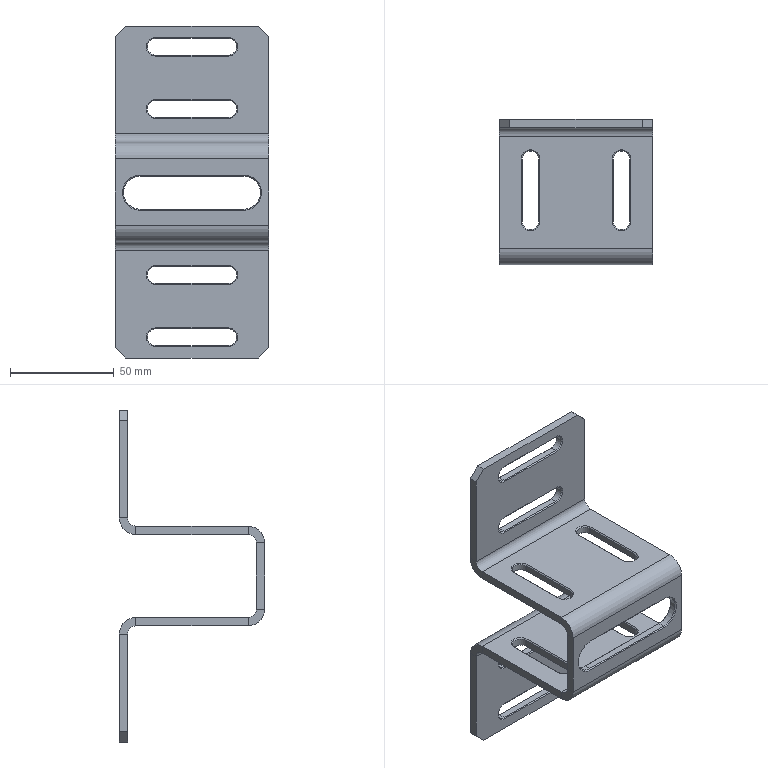Part | STEP file | mocowanie | 1 solid | 142 faces | box 74 x 70 x 160 mm | volume 69052 mm3 | plane 84 | cone 32 | cylinder 26 | commonest cylinder face diameters 8 x20 16 x6